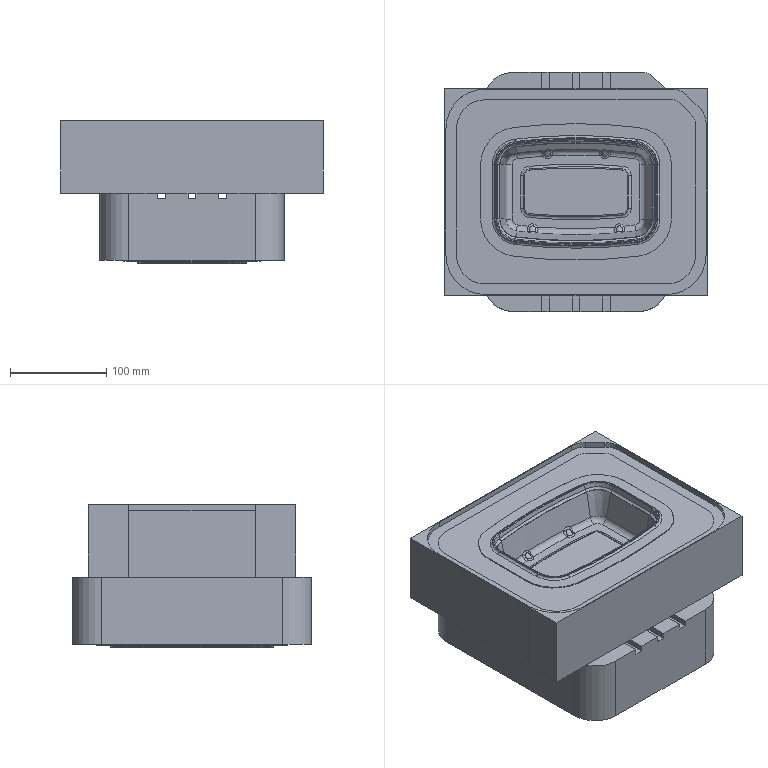NC program | NX | posted with a generic post | part box 272.387 x 248.388 x 148.5 mm
Lines 108276 to 108330 of 133013:
(DRILLING , TOOL : V2.0)
N216538 M6
N216540 G53
N216542 G17 G0 G90 X-44.926 Y59.638 S2000 M3 M8
N216544 G43 Z133. H0
N216546 G94 G81 G98 Z68.707 F150. R73.707
N216548 X-19.206 Y61.214
N216550 X6.561 Y61.525
N216552 X32.312 Y60.57
N216554 X57.985 Y58.35
N216556 X81.363 Y49.096
N216558 X89.966 Y25.612
N216560 Y-0.159
N216562 Y-25.93
N216564 X81.33 Y-49.387
N216566 X57.83 Y-58.367
N216568 X32.157 Y-60.579
N216570 X6.406 Y-61.527
N216572 X-19.361 Y-61.209
N216574 X-45.08 Y-59.625
N216576 X-70.541 Y-56.051
N216578 X-88.17 Y-38.369
N216580 X-89.966 Y-12.808
N216582 Y12.963
N216584 X-88.116 Y38.514
N216586 X-70.395 Y56.105
N216588 X-60. Y32. Z29.51 R34.51
N216590 Y0.
N216592 X-50.48 Z31.005 R36.005
N216594 X-30.
N216596 Y21.151
N216598 Y32. Z29.51 R34.51
N216600 X0. Y22.08 Z31.005 R36.005
N216602 Y32. Z29.51 R34.51
N216604 X30.
N216606 X60.
N216608 X30. Y21.151 Z31.005 R36.005
N216610 Y0.
N216612 X50.48
N216614 X60. Z29.51 R34.51
N216616 Y-32.
N216618 X30.
N216620 Y-21.151 Z31.005 R36.005
N216622 X0. Y-32. Z29.51 R34.51
N216624 Y-22.08 Z31.005 R36.005
N216626 Y0.
N216628 X-30. Y-21.151
N216630 Y-32. Z29.51 R34.51
N216632 X-60.
N216634 G80
N216636 G0 X-60. Y-32. Z133.
N216638 M9
N216640 M5